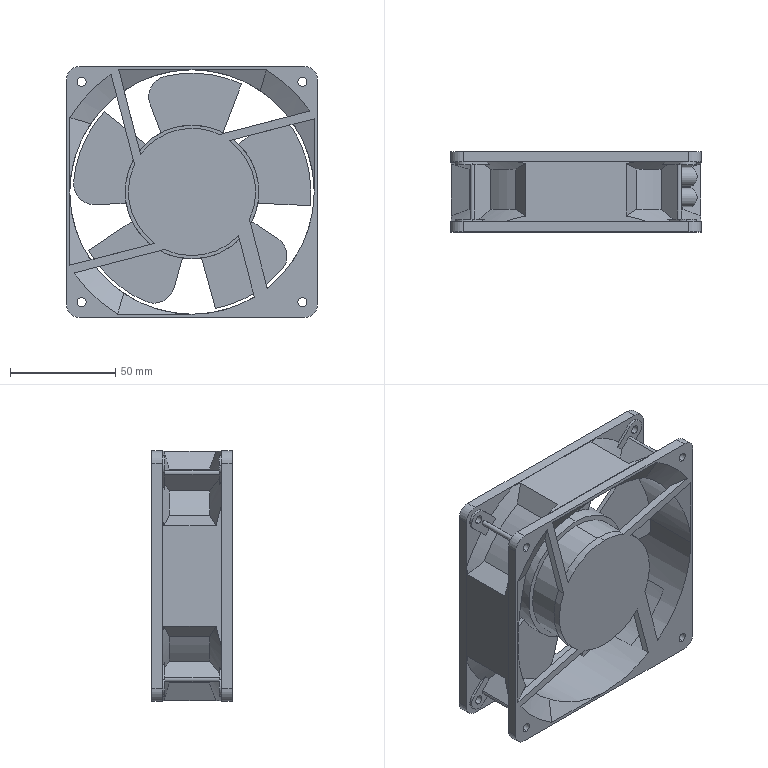Part | SolidWorks | features BaseBody 1 | 1 solid | 221 faces | box 119.126 x 38.1 x 119.126 mm | volume 190423 mm3 | plane 107 | cylinder 87 | cone 27 | commonest cylinder face diameters 4.293 x16 9.53 x12 11.913 x8 116.743 x8 19.963 x7 2.286 x6